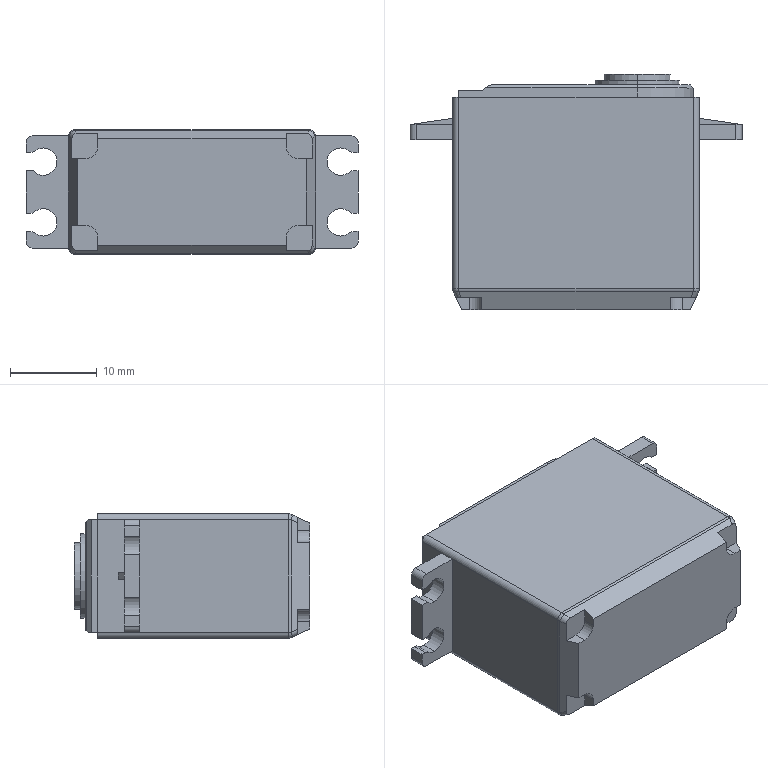Part | SolidWorks | features ICE 14, RevCut 4, Fillet 2, Rib 2, Chamfer 1, Extrusion 1, Revolution 1, Scale 1 | 1 solid | 117 faces | box 38.29 x 27.125 x 14.35 mm | volume 10479 mm3 | plane 65 | cylinder 47 | sphere 4 | cone 1 | commonest cylinder face diameters 1.4 x24 3.15 x12 2.8 x4 3.1 x2 7.7 x2 9.8 x2